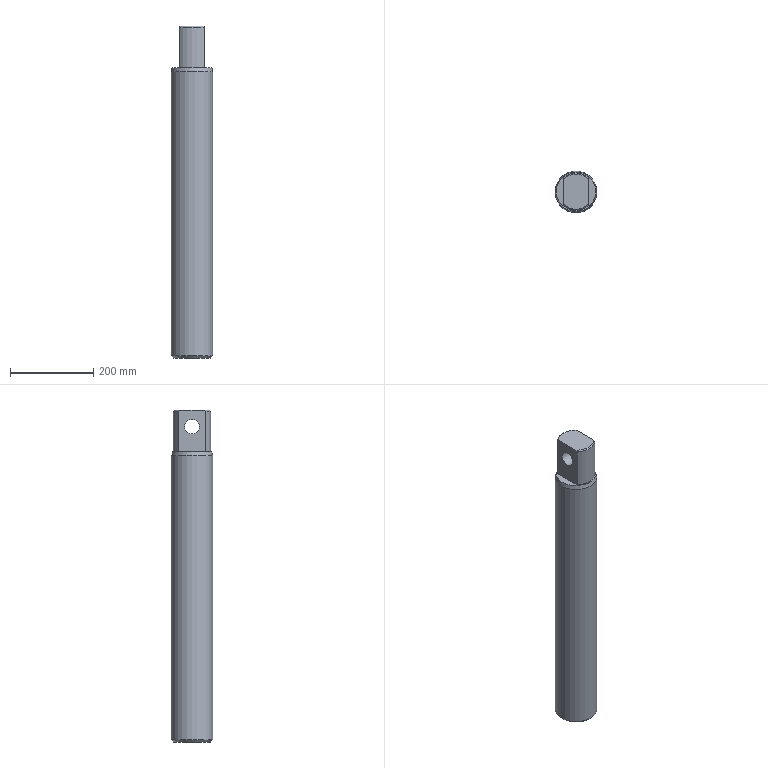Part | NX | features 护帮千斤顶活塞 2 | 1 solid | 13 faces | box 100 x 100 x 798 mm | volume 5913177 mm3 | plane 5 | cylinder 4 | cone 4 | commonest cylinder face diameters 90 x2 35 x1 100 x1
STEP:
#1=CARTESIAN_POINT('',(-30.,33.541,795.));
#2=VERTEX_POINT('',#1);
#3=CARTESIAN_POINT('',(-30.,33.541,698.));
#4=VERTEX_POINT('',#3);
#5=CARTESIAN_POINT('',(-30.,33.541,798.));
#6=DIRECTION('',(0.,0.,-1.));
#7=VECTOR('',#6,1000.);
#8=LINE('',#5,#7);
#9=EDGE_CURVE('',#2,#4,#8,.T.);
#10=ORIENTED_EDGE('',*,*,#9,.F.);
#11=CARTESIAN_POINT('',(30.,33.541,795.));
#12=VERTEX_POINT('',#11);
#13=CARTESIAN_POINT('',(0.,0.,795.));
#14=DIRECTION('',(0.,0.,1.));
#15=DIRECTION('',(1.,0.,0.));
#16=AXIS2_PLACEMENT_3D('',#13,#14,#15);
#17=CIRCLE('',#16,45.);
#18=EDGE_CURVE('',#2,#12,#17,.F.);
#19=ORIENTED_EDGE('',*,*,#18,.T.);
#20=CARTESIAN_POINT('',(30.,33.541,698.));
#21=VERTEX_POINT('',#20);
#22=CARTESIAN_POINT('',(30.,33.541,798.));
#23=DIRECTION('',(0.,0.,-1.));
#24=VECTOR('',#23,1000.);
#25=LINE('',#22,#24);
#26=EDGE_CURVE('',#21,#12,#25,.F.);
#27=ORIENTED_EDGE('',*,*,#26,.F.);
#28=CARTESIAN_POINT('',(0.,0.,698.));
#29=DIRECTION('',(0.,0.,1.));
#30=DIRECTION('',(1.,0.,0.));
#31=AXIS2_PLACEMENT_3D('',#28,#29,#30);
#32=CIRCLE('',#31,45.);
#33=EDGE_CURVE('',#21,#4,#32,.T.);
#34=ORIENTED_EDGE('',*,*,#33,.T.);
#35=EDGE_LOOP('',(#10,#19,#27,#34));
#36=FACE_BOUND('',#35,.T.);
#37=CARTESIAN_POINT('',(0.,0.,798.));
#38=DIRECTION('',(0.,0.,-1.));
#39=DIRECTION('',(-1.,0.,0.));
#40=AXIS2_PLACEMENT_3D('',#37,#38,#39);
#41=CYLINDRICAL_SURFACE('',#40,45.);
#42=ADVANCED_FACE('',(#36),#41,.T.);
#43=CARTESIAN_POINT('',(-30.,-33.541,698.));
#44=VERTEX_POINT('',#43);
#45=CARTESIAN_POINT('',(-30.,-33.541,795.));
#46=VERTEX_POINT('',#45);
#47=CARTESIAN_POINT('',(-30.,-33.541,798.));
#48=DIRECTION('',(0.,0.,-1.));
#49=VECTOR('',#48,1000.);
#50=LINE('',#47,#49);
#51=EDGE_CURVE('',#44,#46,#50,.F.);
#52=ORIENTED_EDGE('',*,*,#51,.F.);
#53=CARTESIAN_POINT('',(30.,-33.541,698.));
#54=VERTEX_POINT('',#53);
#55=CARTESIAN_POINT('',(0.,0.,698.));
#56=DIRECTION('',(0.,0.,1.));
#57=DIRECTION('',(1.,0.,0.));
#58=AXIS2_PLACEMENT_3D('',#55,#56,#57);
#59=CIRCLE('',#58,45.);
#60=EDGE_CURVE('',#44,#54,#59,.T.);
#61=ORIENTED_EDGE('',*,*,#60,.T.);
#62=CARTESIAN_POINT('',(30.,-33.541,795.));
#63=VERTEX_POINT('',#62);
#64=CARTESIAN_POINT('',(30.,-33.541,798.));
#65=DIRECTION('',(0.,0.,-1.));
#66=VECTOR('',#65,1000.);
#67=LINE('',#64,#66);
#68=EDGE_CURVE('',#63,#54,#67,.T.);
#69=ORIENTED_EDGE('',*,*,#68,.F.);
#70=CARTESIAN_POINT('',(0.,0.,795.));
#71=DIRECTION('',(0.,0.,1.));
#72=DIRECTION('',(1.,0.,0.));
#73=AXIS2_PLACEMENT_3D('',#70,#71,#72);
#74=CIRCLE('',#73,45.);
#75=EDGE_CURVE('',#63,#46,#74,.F.);
#76=ORIENTED_EDGE('',*,*,#75,.T.);
#77=EDGE_LOOP('',(#52,#61,#69,#76));
#78=FACE_BOUND('',#77,.T.);
#79=CARTESIAN_POINT('',(0.,0.,798.));
#80=DIRECTION('',(0.,0.,-1.));
#81=DIRECTION('',(-1.,0.,0.));
#82=AXIS2_PLACEMENT_3D('',#79,#80,#81);
#83=CYLINDRICAL_SURFACE('',#82,45.);
#84=ADVANCED_FACE('',(#78),#83,.T.);
#85=CARTESIAN_POINT('',(30.,29.394,798.));
#86=VERTEX_POINT('',#85);
#87=CARTESIAN_POINT('',(-30.,29.394,798.));
#88=VERTEX_POINT('',#87);
#89=CARTESIAN_POINT('',(0.,0.,798.));
#90=DIRECTION('',(0.,0.,1.));
#91=DIRECTION('',(1.,0.,0.));
#92=AXIS2_PLACEMENT_3D('',#89,#90,#91);
#93=CIRCLE('',#92,42.);
#94=EDGE_CURVE('',#86,#88,#93,.T.);
#95=ORIENTED_EDGE('',*,*,#94,.T.);
#96=CARTESIAN_POINT('',(-30.,-29.394,798.));
#97=VERTEX_POINT('',#96);
#98=CARTESIAN_POINT('',(-30.,50.33,798.));
#99=DIRECTION('',(0.,-1.,0.));
#100=VECTOR('',#99,1000.);
#101=LINE('',#98,#100);
#102=EDGE_CURVE('',#88,#97,#101,.T.);
#103=ORIENTED_EDGE('',*,*,#102,.T.);
#104=CARTESIAN_POINT('',(30.,-29.394,798.));
#105=VERTEX_POINT('',#104);
#106=CARTESIAN_POINT('',(0.,0.,798.));
#107=DIRECTION('',(0.,0.,1.));
#108=DIRECTION('',(1.,0.,0.));
#109=AXIS2_PLACEMENT_3D('',#106,#107,#108);
#110=CIRCLE('',#109,42.);
#111=EDGE_CURVE('',#97,#105,#110,.T.);
#112=ORIENTED_EDGE('',*,*,#111,.T.);
#113=CARTESIAN_POINT('',(30.,50.33,798.));
#114=DIRECTION('',(0.,1.,0.));
#115=VECTOR('',#114,1000.);
#116=LINE('',#113,#115);
#117=EDGE_CURVE('',#105,#86,#116,.T.);
#118=ORIENTED_EDGE('',*,*,#117,.T.);
#119=EDGE_LOOP('',(#95,#103,#112,#118));
#120=FACE_BOUND('',#119,.T.);
#121=CARTESIAN_POINT('',(0.,0.,798.));
#122=DIRECTION('',(0.,0.,1.));
#123=DIRECTION('',(1.,0.,0.));
#124=AXIS2_PLACEMENT_3D('',#121,#122,#123);
#125=PLANE('',#124);
#126=ADVANCED_FACE('',(#120),#125,.T.);
#127=ORIENTED_EDGE('',*,*,#18,.F.);
#128=CARTESIAN_POINT('',(-30.,33.541,795.));
#129=CARTESIAN_POINT('',(-30.,32.174,796.019));
#130=CARTESIAN_POINT('',(-30.,30.793,797.021));
#131=CARTESIAN_POINT('',(-30.,29.394,798.));
#132=B_SPLINE_CURVE_WITH_KNOTS('',3,(#128,#129,#130,#131),.UNSPECIFIED.,.F.,.F.,(4,4),(0.08142,0.08654),.UNSPECIFIED.);
#133=EDGE_CURVE('',#2,#88,#132,.T.);
#134=ORIENTED_EDGE('',*,*,#133,.T.);
#135=ORIENTED_EDGE('',*,*,#94,.F.);
#136=CARTESIAN_POINT('',(30.,29.394,798.));
#137=CARTESIAN_POINT('',(30.,30.79,797.023));
#138=CARTESIAN_POINT('',(30.,32.172,796.021));
#139=CARTESIAN_POINT('',(30.,33.541,795.));
#140=B_SPLINE_CURVE_WITH_KNOTS('',3,(#136,#137,#138,#139),.UNSPECIFIED.,.F.,.F.,(4,4),(0.1511,0.1562),.UNSPECIFIED.);
#141=EDGE_CURVE('',#86,#12,#140,.T.);
#142=ORIENTED_EDGE('',*,*,#141,.T.);
#143=EDGE_LOOP('',(#127,#134,#135,#142));
#144=FACE_BOUND('',#143,.T.);
#145=CARTESIAN_POINT('',(0.,0.,798.));
#146=DIRECTION('',(0.,0.,-1.));
#147=DIRECTION('',(-1.,0.,0.));
#148=AXIS2_PLACEMENT_3D('',#145,#146,#147);
#149=CONICAL_SURFACE('',#148,42.,0.7854);
#150=ADVANCED_FACE('',(#144),#149,.T.);
#151=ORIENTED_EDGE('',*,*,#111,.F.);
#152=CARTESIAN_POINT('',(-30.,-29.394,798.));
#153=CARTESIAN_POINT('',(-30.,-30.79,797.023));
#154=CARTESIAN_POINT('',(-30.,-32.172,796.021));
#155=CARTESIAN_POINT('',(-30.,-33.541,795.));
#156=B_SPLINE_CURVE_WITH_KNOTS('',3,(#152,#153,#154,#155),.UNSPECIFIED.,.F.,.F.,(4,4),(0.1511,0.1562),.UNSPECIFIED.);
#157=EDGE_CURVE('',#97,#46,#156,.T.);
#158=ORIENTED_EDGE('',*,*,#157,.T.);
#159=ORIENTED_EDGE('',*,*,#75,.F.);
#160=CARTESIAN_POINT('',(30.,-33.541,795.));
#161=CARTESIAN_POINT('',(30.,-32.174,796.019));
#162=CARTESIAN_POINT('',(30.,-30.793,797.021));
#163=CARTESIAN_POINT('',(30.,-29.394,798.));
#164=B_SPLINE_CURVE_WITH_KNOTS('',3,(#160,#161,#162,#163),.UNSPECIFIED.,.F.,.F.,(4,4),(0.08142,0.08654),.UNSPECIFIED.);
#165=EDGE_CURVE('',#63,#105,#164,.T.);
#166=ORIENTED_EDGE('',*,*,#165,.T.);
#167=EDGE_LOOP('',(#151,#158,#159,#166));
#168=FACE_BOUND('',#167,.T.);
#169=CARTESIAN_POINT('',(0.,0.,798.));
#170=DIRECTION('',(0.,0.,-1.));
#171=DIRECTION('',(-1.,0.,0.));
#172=AXIS2_PLACEMENT_3D('',#169,#170,#171);
#173=CONICAL_SURFACE('',#172,42.,0.7854);
#174=ADVANCED_FACE('',(#168),#173,.T.);
#175=CARTESIAN_POINT('',(-30.,50.33,698.));
#176=DIRECTION('',(0.,-1.,0.));
#177=VECTOR('',#176,1000.);
#178=LINE('',#175,#177);
#179=EDGE_CURVE('',#4,#44,#178,.T.);
#180=ORIENTED_EDGE('',*,*,#179,.F.);
#181=ORIENTED_EDGE('',*,*,#33,.F.);
#182=CARTESIAN_POINT('',(30.,50.33,698.));
#183=DIRECTION('',(0.,1.,0.));
#184=VECTOR('',#183,1000.);
#185=LINE('',#182,#184);
#186=EDGE_CURVE('',#54,#21,#185,.T.);
#187=ORIENTED_EDGE('',*,*,#186,.F.);
#188=ORIENTED_EDGE('',*,*,#60,.F.);
#189=EDGE_LOOP('',(#180,#181,#187,#188));
#190=FACE_BOUND('',#189,.T.);
#191=CARTESIAN_POINT('',(47.691,0.,698.));
#192=VERTEX_POINT('',#191);
#193=CARTESIAN_POINT('',(0.,0.,698.));
#194=DIRECTION('',(0.,0.,1.));
#195=DIRECTION('',(1.,0.,0.));
#196=AXIS2_PLACEMENT_3D('',#193,#194,#195);
#197=CIRCLE('',#196,47.691);
#198=EDGE_CURVE('',#192,#192,#197,.T.);
#199=ORIENTED_EDGE('',*,*,#198,.T.);
#200=EDGE_LOOP('',(#199));
#201=FACE_BOUND('',#200,.T.);
#202=CARTESIAN_POINT('',(0.,0.,698.));
#203=DIRECTION('',(0.,0.,1.));
#204=DIRECTION('',(1.,0.,0.));
#205=AXIS2_PLACEMENT_3D('',#202,#203,#204);
#206=PLANE('',#205);
#207=ADVANCED_FACE('',(#190,#201),#206,.T.);
#208=CARTESIAN_POINT('',(50.,0.,5.));
#209=VERTEX_POINT('',#208);
#210=CARTESIAN_POINT('',(0.,0.,5.));
#211=DIRECTION('',(0.,0.,1.));
#212=DIRECTION('',(1.,0.,0.));
#213=AXIS2_PLACEMENT_3D('',#210,#211,#212);
#214=CIRCLE('',#213,50.);
#215=EDGE_CURVE('',#209,#209,#214,.T.);
#216=ORIENTED_EDGE('',*,*,#215,.T.);
#217=EDGE_LOOP('',(#216));
#218=FACE_BOUND('',#217,.T.);
#219=CARTESIAN_POINT('',(50.,0.,688.));
#220=VERTEX_POINT('',#219);
#221=CARTESIAN_POINT('',(0.,0.,688.));
#222=DIRECTION('',(0.,0.,1.));
#223=DIRECTION('',(1.,0.,0.));
#224=AXIS2_PLACEMENT_3D('',#221,#222,#223);
#225=CIRCLE('',#224,50.);
#226=EDGE_CURVE('',#220,#220,#225,.F.);
#227=ORIENTED_EDGE('',*,*,#226,.T.);
#228=EDGE_LOOP('',(#227));
#229=FACE_BOUND('',#228,.T.);
#230=CARTESIAN_POINT('',(0.,0.,698.));
#231=DIRECTION('',(0.,0.,-1.));
#232=DIRECTION('',(-1.,0.,0.));
#233=AXIS2_PLACEMENT_3D('',#230,#231,#232);
#234=CYLINDRICAL_SURFACE('',#233,50.);
#235=ADVANCED_FACE('',(#218,#229),#234,.T.);
#236=CARTESIAN_POINT('',(45.,0.,0.));
#237=VERTEX_POINT('',#236);
#238=CARTESIAN_POINT('',(0.,0.,0.));
#239=DIRECTION('',(0.,0.,1.));
#240=DIRECTION('',(1.,0.,0.));
#241=AXIS2_PLACEMENT_3D('',#238,#239,#240);
#242=CIRCLE('',#241,45.);
#243=EDGE_CURVE('',#237,#237,#242,.F.);
#244=ORIENTED_EDGE('',*,*,#243,.T.);
#245=EDGE_LOOP('',(#244));
#246=FACE_BOUND('',#245,.T.);
#247=CARTESIAN_POINT('',(0.,0.,0.));
#248=DIRECTION('',(0.,0.,1.));
#249=DIRECTION('',(1.,0.,0.));
#250=AXIS2_PLACEMENT_3D('',#247,#248,#249);
#251=PLANE('',#250);
#252=ADVANCED_FACE('',(#246),#251,.F.);
#253=ORIENTED_EDGE('',*,*,#226,.F.);
#254=EDGE_LOOP('',(#253));
#255=FACE_BOUND('',#254,.T.);
#256=ORIENTED_EDGE('',*,*,#198,.F.);
#257=EDGE_LOOP('',(#256));
#258=FACE_BOUND('',#257,.T.);
#259=CARTESIAN_POINT('',(0.,0.,698.));
#260=DIRECTION('',(0.,0.,-1.));
#261=DIRECTION('',(-1.,0.,0.));
#262=AXIS2_PLACEMENT_3D('',#259,#260,#261);
#263=CONICAL_SURFACE('',#262,47.691,0.2269);
#264=ADVANCED_FACE('',(#255,#258),#263,.T.);
#265=ORIENTED_EDGE('',*,*,#243,.F.);
#266=EDGE_LOOP('',(#265));
#267=FACE_BOUND('',#266,.T.);
#268=ORIENTED_EDGE('',*,*,#215,.F.);
#269=EDGE_LOOP('',(#268));
#270=FACE_BOUND('',#269,.T.);
#271=CARTESIAN_POINT('',(0.,0.,5.));
#272=DIRECTION('',(0.,0.,1.));
#273=DIRECTION('',(1.,0.,0.));
#274=AXIS2_PLACEMENT_3D('',#271,#272,#273);
#275=CONICAL_SURFACE('',#274,50.,0.7854);
#276=ADVANCED_FACE('',(#267,#270),#275,.T.);
#277=CARTESIAN_POINT('',(30.,17.5,758.));
#278=VERTEX_POINT('',#277);
#279=CARTESIAN_POINT('',(30.,0.,758.));
#280=DIRECTION('',(1.,0.,0.));
#281=DIRECTION('',(0.,1.,0.));
#282=AXIS2_PLACEMENT_3D('',#279,#280,#281);
#283=CIRCLE('',#282,17.5);
#284=EDGE_CURVE('',#278,#278,#283,.F.);
#285=ORIENTED_EDGE('',*,*,#284,.T.);
#286=EDGE_LOOP('',(#285));
#287=FACE_BOUND('',#286,.T.);
#288=ORIENTED_EDGE('',*,*,#68,.T.);
#289=ORIENTED_EDGE('',*,*,#186,.T.);
#290=ORIENTED_EDGE('',*,*,#26,.T.);
#291=ORIENTED_EDGE('',*,*,#141,.F.);
#292=ORIENTED_EDGE('',*,*,#117,.F.);
#293=ORIENTED_EDGE('',*,*,#165,.F.);
#294=EDGE_LOOP('',(#288,#289,#290,#291,#292,#293));
#295=FACE_BOUND('',#294,.T.);
#296=CARTESIAN_POINT('',(30.,50.33,698.));
#297=DIRECTION('',(1.,0.,0.));
#298=DIRECTION('',(0.,1.,0.));
#299=AXIS2_PLACEMENT_3D('',#296,#297,#298);
#300=PLANE('',#299);
#301=ADVANCED_FACE('',(#287,#295),#300,.T.);
#302=CARTESIAN_POINT('',(-30.,-17.5,758.));
#303=VERTEX_POINT('',#302);
#304=CARTESIAN_POINT('',(-30.,0.,758.));
#305=DIRECTION('',(-1.,0.,0.));
#306=DIRECTION('',(0.,-1.,0.));
#307=AXIS2_PLACEMENT_3D('',#304,#305,#306);
#308=CIRCLE('',#307,17.5);
#309=EDGE_CURVE('',#303,#303,#308,.F.);
#310=ORIENTED_EDGE('',*,*,#309,.T.);
#311=EDGE_LOOP('',(#310));
#312=FACE_BOUND('',#311,.T.);
#313=ORIENTED_EDGE('',*,*,#9,.T.);
#314=ORIENTED_EDGE('',*,*,#179,.T.);
#315=ORIENTED_EDGE('',*,*,#51,.T.);
#316=ORIENTED_EDGE('',*,*,#157,.F.);
#317=ORIENTED_EDGE('',*,*,#102,.F.);
#318=ORIENTED_EDGE('',*,*,#133,.F.);
#319=EDGE_LOOP('',(#313,#314,#315,#316,#317,#318));
#320=FACE_BOUND('',#319,.T.);
#321=CARTESIAN_POINT('',(-30.,50.33,698.));
#322=DIRECTION('',(-1.,0.,0.));
#323=DIRECTION('',(0.,-1.,0.));
#324=AXIS2_PLACEMENT_3D('',#321,#322,#323);
#325=PLANE('',#324);
#326=ADVANCED_FACE('',(#312,#320),#325,.T.);
#327=ORIENTED_EDGE('',*,*,#284,.F.);
#328=EDGE_LOOP('',(#327));
#329=FACE_BOUND('',#328,.T.);
#330=ORIENTED_EDGE('',*,*,#309,.F.);
#331=EDGE_LOOP('',(#330));
#332=FACE_BOUND('',#331,.T.);
#333=CARTESIAN_POINT('',(-60.,0.,758.));
#334=DIRECTION('',(1.,0.,0.));
#335=DIRECTION('',(0.,0.,-1.));
#336=AXIS2_PLACEMENT_3D('',#333,#334,#335);
#337=CYLINDRICAL_SURFACE('',#336,17.5);
#338=ADVANCED_FACE('',(#329,#332),#337,.F.);
#339=CLOSED_SHELL('',(#42,#84,#126,#150,#174,#207,#235,#252,#264,#276,#301,#326,#338));
#340=MANIFOLD_SOLID_BREP('',#339);
#341=(LENGTH_UNIT()NAMED_UNIT(*)SI_UNIT(.MILLI.,.METRE.));
#342=UNCERTAINTY_MEASURE_WITH_UNIT(LENGTH_MEASURE(0.0508),#341,'','');
#343=(NAMED_UNIT(*)PLANE_ANGLE_UNIT()SI_UNIT($,.RADIAN.));
#344=(NAMED_UNIT(*)SI_UNIT($,.STERADIAN.)SOLID_ANGLE_UNIT());
#345=(GEOMETRIC_REPRESENTATION_CONTEXT(3)GLOBAL_UNCERTAINTY_ASSIGNED_CONTEXT((#342))GLOBAL_UNIT_ASSIGNED_CONTEXT((#341,#343,#344))REPRESENTATION_CONTEXT('',''));
#346=ADVANCED_BREP_SHAPE_REPRESENTATION('',(#340),#345);